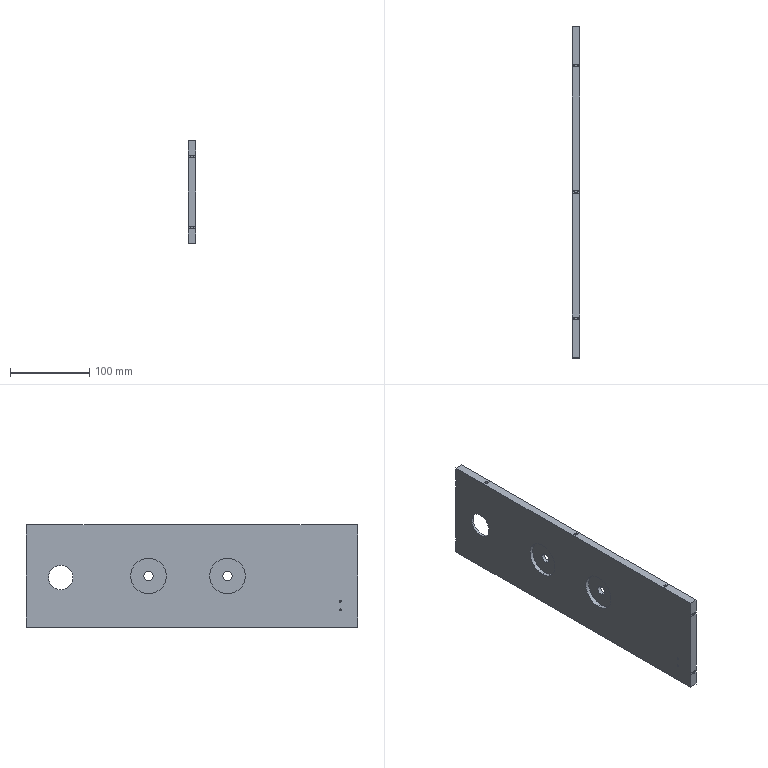Part | SolidWorks | features BaseBody 1 | 1 solid | 80 faces | box 10 x 420 x 130 mm | volume 507586 mm3 | cylinder 53 | plane 21 | cone 6 | commonest cylinder face diameters 10 x20 3.3 x19 2.5 x4 12 x4 45 x4 31 x2